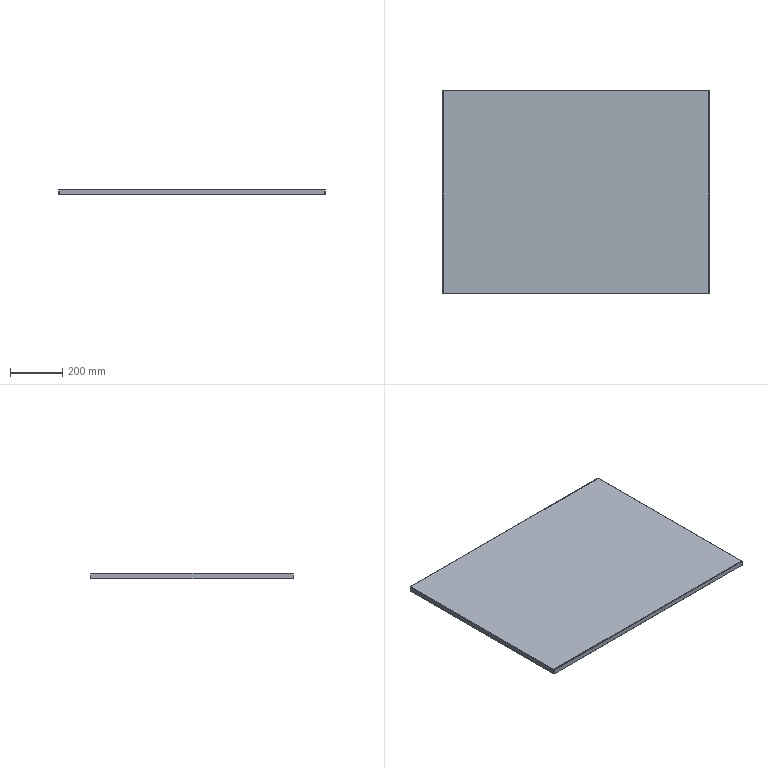Part | STEP file | X77-03016 | 1 solid | 38 faces | box 1018 x 778 x 20 mm | volume 1283744 mm3 | plane 22 | spline 8 | cylinder 8 | commonest cylinder face diameters 1.473 x4 4.473 x4
STEP:
#1=CARTESIAN_POINT('',(23.994,-5274.803,-1.5));
#2=VERTEX_POINT('',#1);
#3=CARTESIAN_POINT('',(1037.521,-5274.803,-1.5));
#4=VERTEX_POINT('',#3);
#5=CARTESIAN_POINT('',(23.964,-5274.803,-1.5));
#6=DIRECTION('',(1.,0.,0.));
#7=VECTOR('',#6,1000.);
#8=LINE('',#5,#7);
#9=EDGE_CURVE('',#2,#4,#8,.T.);
#10=ORIENTED_EDGE('',*,*,#9,.F.);
#11=CARTESIAN_POINT('',(23.994,-4501.276,-1.5));
#12=VERTEX_POINT('',#11);
#13=CARTESIAN_POINT('',(23.994,-4501.247,-1.5));
#14=DIRECTION('',(0.,-1.,0.));
#15=VECTOR('',#14,1000.);
#16=LINE('',#13,#15);
#17=EDGE_CURVE('',#12,#2,#16,.T.);
#18=ORIENTED_EDGE('',*,*,#17,.F.);
#19=CARTESIAN_POINT('',(1037.521,-4501.276,-1.5));
#20=VERTEX_POINT('',#19);
#21=CARTESIAN_POINT('',(1037.55,-4501.276,-1.5));
#22=DIRECTION('',(-1.,0.,0.));
#23=VECTOR('',#22,1000.);
#24=LINE('',#21,#23);
#25=EDGE_CURVE('',#20,#12,#24,.T.);
#26=ORIENTED_EDGE('',*,*,#25,.F.);
#27=CARTESIAN_POINT('',(1037.521,-5274.833,-1.5));
#28=DIRECTION('',(0.,1.,0.));
#29=VECTOR('',#28,1000.);
#30=LINE('',#27,#29);
#31=EDGE_CURVE('',#4,#20,#30,.T.);
#32=ORIENTED_EDGE('',*,*,#31,.F.);
#33=EDGE_LOOP('',(#10,#18,#26,#32));
#34=FACE_OUTER_BOUND('',#33,.T.);
#35=CARTESIAN_POINT('',(23.257,-5275.54,-1.5));
#36=DIRECTION('',(0.,0.,1.));
#37=DIRECTION('',(1.,0.,0.));
#38=AXIS2_PLACEMENT_3D('',#35,#36,#37);
#39=PLANE('',#38);
#40=ADVANCED_FACE('',(#34),#39,.F.);
#41=CARTESIAN_POINT('',(23.994,-4501.276,0.));
#42=VERTEX_POINT('',#41);
#43=CARTESIAN_POINT('',(23.994,-5274.803,0.));
#44=VERTEX_POINT('',#43);
#45=CARTESIAN_POINT('',(23.994,-4501.247,0.));
#46=DIRECTION('',(0.,-1.,0.));
#47=VECTOR('',#46,1000.);
#48=LINE('',#45,#47);
#49=EDGE_CURVE('',#42,#44,#48,.T.);
#50=ORIENTED_EDGE('',*,*,#49,.T.);
#51=CARTESIAN_POINT('',(1037.521,-5274.803,0.));
#52=VERTEX_POINT('',#51);
#53=CARTESIAN_POINT('',(23.964,-5274.803,0.));
#54=DIRECTION('',(1.,0.,0.));
#55=VECTOR('',#54,1000.);
#56=LINE('',#53,#55);
#57=EDGE_CURVE('',#44,#52,#56,.T.);
#58=ORIENTED_EDGE('',*,*,#57,.T.);
#59=CARTESIAN_POINT('',(1037.521,-4501.276,0.));
#60=VERTEX_POINT('',#59);
#61=CARTESIAN_POINT('',(1037.521,-5274.833,0.));
#62=DIRECTION('',(0.,1.,0.));
#63=VECTOR('',#62,1000.);
#64=LINE('',#61,#63);
#65=EDGE_CURVE('',#52,#60,#64,.T.);
#66=ORIENTED_EDGE('',*,*,#65,.T.);
#67=CARTESIAN_POINT('',(1037.55,-4501.276,0.));
#68=DIRECTION('',(-1.,0.,0.));
#69=VECTOR('',#68,1000.);
#70=LINE('',#67,#69);
#71=EDGE_CURVE('',#60,#42,#70,.T.);
#72=ORIENTED_EDGE('',*,*,#71,.T.);
#73=EDGE_LOOP('',(#50,#58,#66,#72));
#74=FACE_OUTER_BOUND('',#73,.T.);
#75=CARTESIAN_POINT('',(23.257,-5275.54,0.));
#76=DIRECTION('',(0.,0.,1.));
#77=DIRECTION('',(1.,0.,0.));
#78=AXIS2_PLACEMENT_3D('',#75,#76,#77);
#79=PLANE('',#78);
#80=ADVANCED_FACE('',(#74),#79,.T.);
#81=CARTESIAN_POINT('',(21.757,-5274.833,-2.237));
#82=VERTEX_POINT('',#81);
#83=CARTESIAN_POINT('',(23.257,-5274.833,-2.237));
#84=VERTEX_POINT('',#83);
#85=CARTESIAN_POINT('',(23.257,-5274.833,-2.237));
#86=DIRECTION('',(1.,0.,0.));
#87=VECTOR('',#86,1000.);
#88=LINE('',#85,#87);
#89=EDGE_CURVE('',#82,#84,#88,.T.);
#90=ORIENTED_EDGE('',*,*,#89,.T.);
#91=CARTESIAN_POINT('',(23.994,-5274.803,-1.5));
#92=CARTESIAN_POINT('',(23.801,-5274.808,-1.5));
#93=CARTESIAN_POINT('',(23.609,-5274.813,-1.579));
#94=CARTESIAN_POINT('',(23.337,-5274.823,-1.852));
#95=CARTESIAN_POINT('',(23.257,-5274.828,-2.044));
#96=CARTESIAN_POINT('',(23.257,-5274.833,-2.237));
#97=B_SPLINE_CURVE_WITH_KNOTS('',3,(#91,#92,#93,#94,#95,#96),.UNSPECIFIED.,.F.,.F.,(4,2,4),(0.,0.5,1.),.UNSPECIFIED.);
#98=EDGE_CURVE('',#2,#84,#97,.T.);
#99=ORIENTED_EDGE('',*,*,#98,.F.);
#100=CARTESIAN_POINT('',(23.994,-5274.803,-1.5));
#101=DIRECTION('',(0.,0.,1.));
#102=VECTOR('',#101,1000.);
#103=LINE('',#100,#102);
#104=EDGE_CURVE('',#2,#44,#103,.T.);
#105=ORIENTED_EDGE('',*,*,#104,.T.);
#106=CARTESIAN_POINT('',(23.994,-5274.803,0.));
#107=CARTESIAN_POINT('',(23.701,-5274.806,0.));
#108=CARTESIAN_POINT('',(23.408,-5274.808,-0.05821));
#109=CARTESIAN_POINT('',(22.867,-5274.813,-0.2823));
#110=CARTESIAN_POINT('',(22.619,-5274.815,-0.4481));
#111=CARTESIAN_POINT('',(22.205,-5274.82,-0.8621));
#112=CARTESIAN_POINT('',(22.04,-5274.823,-1.11));
#113=CARTESIAN_POINT('',(21.815,-5274.828,-1.651));
#114=CARTESIAN_POINT('',(21.757,-5274.83,-1.944));
#115=CARTESIAN_POINT('',(21.757,-5274.833,-2.237));
#116=B_SPLINE_CURVE_WITH_KNOTS('',3,(#106,#107,#108,#109,#110,#111,#112,#113,#114,#115),.UNSPECIFIED.,.F.,.F.,(4,2,2,2,4),(0.,0.25,0.5,0.75,1.),.UNSPECIFIED.);
#117=EDGE_CURVE('',#44,#82,#116,.T.);
#118=ORIENTED_EDGE('',*,*,#117,.T.);
#119=EDGE_LOOP('',(#90,#99,#105,#118));
#120=FACE_OUTER_BOUND('',#119,.T.);
#121=CARTESIAN_POINT('',(23.994,-5274.803,0.015));
#122=CARTESIAN_POINT('',(23.699,-5274.806,0.015));
#123=CARTESIAN_POINT('',(23.405,-5274.808,-0.0436));
#124=CARTESIAN_POINT('',(22.86,-5274.813,-0.2692));
#125=CARTESIAN_POINT('',(22.61,-5274.815,-0.4361));
#126=CARTESIAN_POINT('',(22.193,-5274.82,-0.8529));
#127=CARTESIAN_POINT('',(22.026,-5274.823,-1.103));
#128=CARTESIAN_POINT('',(21.801,-5274.828,-1.647));
#129=CARTESIAN_POINT('',(21.742,-5274.83,-1.942));
#130=CARTESIAN_POINT('',(21.742,-5274.833,-2.237));
#131=CARTESIAN_POINT('',(23.994,-5274.803,0.));
#132=CARTESIAN_POINT('',(23.701,-5274.806,0.));
#133=CARTESIAN_POINT('',(23.408,-5274.808,-0.05821));
#134=CARTESIAN_POINT('',(22.867,-5274.813,-0.2823));
#135=CARTESIAN_POINT('',(22.619,-5274.815,-0.4481));
#136=CARTESIAN_POINT('',(22.205,-5274.82,-0.8621));
#137=CARTESIAN_POINT('',(22.04,-5274.823,-1.11));
#138=CARTESIAN_POINT('',(21.815,-5274.828,-1.651));
#139=CARTESIAN_POINT('',(21.757,-5274.83,-1.944));
#140=CARTESIAN_POINT('',(21.757,-5274.833,-2.237));
#141=CARTESIAN_POINT('',(23.994,-5274.803,-1.5));
#142=CARTESIAN_POINT('',(23.897,-5274.806,-1.5));
#143=CARTESIAN_POINT('',(23.801,-5274.808,-1.519));
#144=CARTESIAN_POINT('',(23.623,-5274.813,-1.593));
#145=CARTESIAN_POINT('',(23.541,-5274.815,-1.648));
#146=CARTESIAN_POINT('',(23.405,-5274.82,-1.784));
#147=CARTESIAN_POINT('',(23.35,-5274.823,-1.866));
#148=CARTESIAN_POINT('',(23.276,-5274.828,-2.044));
#149=CARTESIAN_POINT('',(23.257,-5274.83,-2.14));
#150=CARTESIAN_POINT('',(23.257,-5274.833,-2.237));
#151=CARTESIAN_POINT('',(23.994,-5274.803,-1.515));
#152=CARTESIAN_POINT('',(23.899,-5274.806,-1.515));
#153=CARTESIAN_POINT('',(23.805,-5274.808,-1.534));
#154=CARTESIAN_POINT('',(23.631,-5274.813,-1.606));
#155=CARTESIAN_POINT('',(23.551,-5274.815,-1.66));
#156=CARTESIAN_POINT('',(23.417,-5274.82,-1.793));
#157=CARTESIAN_POINT('',(23.363,-5274.823,-1.873));
#158=CARTESIAN_POINT('',(23.291,-5274.828,-2.048));
#159=CARTESIAN_POINT('',(23.272,-5274.83,-2.142));
#160=CARTESIAN_POINT('',(23.272,-5274.833,-2.237));
#161=B_SPLINE_SURFACE_WITH_KNOTS('',1,3,((#121,#122,#123,#124,#125,#126,#127,#128,#129,#130),(#131,#132,#133,#134,#135,#136,#137,#138,#139,#140),(#141,#142,#143,#144,#145,#146,#147,#148,#149,#150),(#151,#152,#153,#154,#155,#156,#157,#158,#159,#160)),.UNSPECIFIED.,.F.,.F.,.F.,(2,1,1,2),(4,2,2,2,4),(-0.01,0.,1.,1.01),(0.,0.25,0.5,0.75,1.),.UNSPECIFIED.);
#162=ADVANCED_FACE('',(#120),#161,.F.);
#163=ORIENTED_EDGE('',*,*,#49,.F.);
#164=CARTESIAN_POINT('',(21.757,-4501.247,-2.237));
#165=VERTEX_POINT('',#164);
#166=CARTESIAN_POINT('',(21.757,-4501.247,-2.237));
#167=CARTESIAN_POINT('',(21.757,-4501.249,-1.944));
#168=CARTESIAN_POINT('',(21.815,-4501.252,-1.651));
#169=CARTESIAN_POINT('',(22.04,-4501.257,-1.11));
#170=CARTESIAN_POINT('',(22.205,-4501.259,-0.8621));
#171=CARTESIAN_POINT('',(22.619,-4501.264,-0.4481));
#172=CARTESIAN_POINT('',(22.867,-4501.266,-0.2823));
#173=CARTESIAN_POINT('',(23.408,-4501.271,-0.05821));
#174=CARTESIAN_POINT('',(23.701,-4501.274,0.));
#175=CARTESIAN_POINT('',(23.994,-4501.276,0.));
#176=B_SPLINE_CURVE_WITH_KNOTS('',3,(#166,#167,#168,#169,#170,#171,#172,#173,#174,#175),.UNSPECIFIED.,.F.,.F.,(4,2,2,2,4),(0.,0.25,0.5,0.75,1.),.UNSPECIFIED.);
#177=EDGE_CURVE('',#165,#42,#176,.T.);
#178=ORIENTED_EDGE('',*,*,#177,.F.);
#179=CARTESIAN_POINT('',(21.757,-4500.54,-2.237));
#180=DIRECTION('',(0.,1.,0.));
#181=VECTOR('',#180,1000.);
#182=LINE('',#179,#181);
#183=EDGE_CURVE('',#82,#165,#182,.T.);
#184=ORIENTED_EDGE('',*,*,#183,.F.);
#185=ORIENTED_EDGE('',*,*,#117,.F.);
#186=EDGE_LOOP('',(#163,#178,#184,#185));
#187=FACE_OUTER_BOUND('',#186,.T.);
#188=CARTESIAN_POINT('',(23.994,-4501.247,-2.237));
#189=DIRECTION('',(0.,1.,0.));
#190=DIRECTION('',(-1.,0.,0.));
#191=AXIS2_PLACEMENT_3D('',#188,#189,#190);
#192=CYLINDRICAL_SURFACE('',#191,2.237);
#193=ADVANCED_FACE('',(#187),#192,.T.);
#194=CARTESIAN_POINT('',(23.257,-4501.247,-2.237));
#195=VERTEX_POINT('',#194);
#196=CARTESIAN_POINT('',(23.257,-4501.247,-2.237));
#197=CARTESIAN_POINT('',(23.257,-4501.252,-2.044));
#198=CARTESIAN_POINT('',(23.337,-4501.257,-1.852));
#199=CARTESIAN_POINT('',(23.609,-4501.266,-1.579));
#200=CARTESIAN_POINT('',(23.801,-4501.271,-1.5));
#201=CARTESIAN_POINT('',(23.994,-4501.276,-1.5));
#202=B_SPLINE_CURVE_WITH_KNOTS('',3,(#196,#197,#198,#199,#200,#201),.UNSPECIFIED.,.F.,.F.,(4,2,4),(0.,0.5,1.),.UNSPECIFIED.);
#203=EDGE_CURVE('',#195,#12,#202,.T.);
#204=ORIENTED_EDGE('',*,*,#203,.F.);
#205=CARTESIAN_POINT('',(23.257,-4501.247,-2.237));
#206=DIRECTION('',(1.,0.,0.));
#207=VECTOR('',#206,1000.);
#208=LINE('',#205,#207);
#209=EDGE_CURVE('',#165,#195,#208,.T.);
#210=ORIENTED_EDGE('',*,*,#209,.F.);
#211=ORIENTED_EDGE('',*,*,#177,.T.);
#212=CARTESIAN_POINT('',(23.994,-4501.276,-1.5));
#213=DIRECTION('',(0.,0.,1.));
#214=VECTOR('',#213,1000.);
#215=LINE('',#212,#214);
#216=EDGE_CURVE('',#12,#42,#215,.T.);
#217=ORIENTED_EDGE('',*,*,#216,.F.);
#218=EDGE_LOOP('',(#204,#210,#211,#217));
#219=FACE_OUTER_BOUND('',#218,.T.);
#220=CARTESIAN_POINT('',(21.742,-4501.247,-2.237));
#221=CARTESIAN_POINT('',(21.742,-4501.249,-1.942));
#222=CARTESIAN_POINT('',(21.801,-4501.252,-1.647));
#223=CARTESIAN_POINT('',(22.026,-4501.257,-1.103));
#224=CARTESIAN_POINT('',(22.193,-4501.259,-0.8529));
#225=CARTESIAN_POINT('',(22.61,-4501.264,-0.4361));
#226=CARTESIAN_POINT('',(22.86,-4501.266,-0.2692));
#227=CARTESIAN_POINT('',(23.405,-4501.271,-0.0436));
#228=CARTESIAN_POINT('',(23.699,-4501.274,0.015));
#229=CARTESIAN_POINT('',(23.994,-4501.276,0.015));
#230=CARTESIAN_POINT('',(21.757,-4501.247,-2.237));
#231=CARTESIAN_POINT('',(21.757,-4501.249,-1.944));
#232=CARTESIAN_POINT('',(21.815,-4501.252,-1.651));
#233=CARTESIAN_POINT('',(22.04,-4501.257,-1.11));
#234=CARTESIAN_POINT('',(22.205,-4501.259,-0.8621));
#235=CARTESIAN_POINT('',(22.619,-4501.264,-0.4481));
#236=CARTESIAN_POINT('',(22.867,-4501.266,-0.2823));
#237=CARTESIAN_POINT('',(23.408,-4501.271,-0.05821));
#238=CARTESIAN_POINT('',(23.701,-4501.274,0.));
#239=CARTESIAN_POINT('',(23.994,-4501.276,0.));
#240=CARTESIAN_POINT('',(23.257,-4501.247,-2.237));
#241=CARTESIAN_POINT('',(23.257,-4501.249,-2.14));
#242=CARTESIAN_POINT('',(23.276,-4501.252,-2.044));
#243=CARTESIAN_POINT('',(23.35,-4501.257,-1.866));
#244=CARTESIAN_POINT('',(23.405,-4501.259,-1.784));
#245=CARTESIAN_POINT('',(23.541,-4501.264,-1.648));
#246=CARTESIAN_POINT('',(23.623,-4501.266,-1.593));
#247=CARTESIAN_POINT('',(23.801,-4501.271,-1.519));
#248=CARTESIAN_POINT('',(23.897,-4501.274,-1.5));
#249=CARTESIAN_POINT('',(23.994,-4501.276,-1.5));
#250=CARTESIAN_POINT('',(23.272,-4501.247,-2.237));
#251=CARTESIAN_POINT('',(23.272,-4501.249,-2.142));
#252=CARTESIAN_POINT('',(23.291,-4501.252,-2.048));
#253=CARTESIAN_POINT('',(23.363,-4501.257,-1.873));
#254=CARTESIAN_POINT('',(23.417,-4501.259,-1.793));
#255=CARTESIAN_POINT('',(23.551,-4501.264,-1.66));
#256=CARTESIAN_POINT('',(23.631,-4501.266,-1.606));
#257=CARTESIAN_POINT('',(23.805,-4501.271,-1.534));
#258=CARTESIAN_POINT('',(23.899,-4501.274,-1.515));
#259=CARTESIAN_POINT('',(23.994,-4501.276,-1.515));
#260=B_SPLINE_SURFACE_WITH_KNOTS('',1,3,((#220,#221,#222,#223,#224,#225,#226,#227,#228,#229),(#230,#231,#232,#233,#234,#235,#236,#237,#238,#239),(#240,#241,#242,#243,#244,#245,#246,#247,#248,#249),(#250,#251,#252,#253,#254,#255,#256,#257,#258,#259)),.UNSPECIFIED.,.F.,.F.,.F.,(2,1,1,2),(4,2,2,2,4),(-0.01,0.,1.,1.01),(0.,0.25,0.5,0.75,1.),.UNSPECIFIED.);
#261=ADVANCED_FACE('',(#219),#260,.F.);
#262=ORIENTED_EDGE('',*,*,#17,.T.);
#263=ORIENTED_EDGE('',*,*,#98,.T.);
#264=CARTESIAN_POINT('',(23.257,-5275.54,-2.237));
#265=DIRECTION('',(0.,1.,0.));
#266=VECTOR('',#265,1000.);
#267=LINE('',#264,#266);
#268=EDGE_CURVE('',#84,#195,#267,.T.);
#269=ORIENTED_EDGE('',*,*,#268,.T.);
#270=ORIENTED_EDGE('',*,*,#203,.T.);
#271=EDGE_LOOP('',(#262,#263,#269,#270));
#272=FACE_OUTER_BOUND('',#271,.T.);
#273=CARTESIAN_POINT('',(23.994,-4501.247,-2.237));
#274=DIRECTION('',(0.,1.,0.));
#275=DIRECTION('',(-1.,0.,0.));
#276=AXIS2_PLACEMENT_3D('',#273,#274,#275);
#277=CYLINDRICAL_SURFACE('',#276,0.7366);
#278=ADVANCED_FACE('',(#272),#277,.F.);
#279=CARTESIAN_POINT('',(23.257,-5274.833,-20.));
#280=VERTEX_POINT('',#279);
#281=CARTESIAN_POINT('',(21.757,-5274.833,-20.));
#282=VERTEX_POINT('',#281);
#283=CARTESIAN_POINT('',(21.757,-5274.833,-20.));
#284=DIRECTION('',(-1.,0.,0.));
#285=VECTOR('',#284,1000.);
#286=LINE('',#283,#285);
#287=EDGE_CURVE('',#280,#282,#286,.T.);
#288=ORIENTED_EDGE('',*,*,#287,.F.);
#289=CARTESIAN_POINT('',(23.257,-5274.833,-1.5));
#290=DIRECTION('',(0.,0.,-1.));
#291=VECTOR('',#290,1000.);
#292=LINE('',#289,#291);
#293=EDGE_CURVE('',#84,#280,#292,.T.);
#294=ORIENTED_EDGE('',*,*,#293,.F.);
#295=ORIENTED_EDGE('',*,*,#89,.F.);
#296=CARTESIAN_POINT('',(21.757,-5274.833,-1.5));
#297=DIRECTION('',(0.,0.,1.));
#298=VECTOR('',#297,1000.);
#299=LINE('',#296,#298);
#300=EDGE_CURVE('',#282,#82,#299,.T.);
#301=ORIENTED_EDGE('',*,*,#300,.F.);
#302=EDGE_LOOP('',(#288,#294,#295,#301));
#303=FACE_OUTER_BOUND('',#302,.T.);
#304=CARTESIAN_POINT('',(23.257,-5274.833,-1.5));
#305=DIRECTION('',(0.,-1.,0.));
#306=DIRECTION('',(0.,0.,-1.));
#307=AXIS2_PLACEMENT_3D('',#304,#305,#306);
#308=PLANE('',#307);
#309=ADVANCED_FACE('',(#303),#308,.T.);
#310=CARTESIAN_POINT('',(21.757,-4501.247,-20.));
#311=VERTEX_POINT('',#310);
#312=CARTESIAN_POINT('',(21.757,-4501.247,-1.5));
#313=DIRECTION('',(0.,0.,1.));
#314=VECTOR('',#313,1000.);
#315=LINE('',#312,#314);
#316=EDGE_CURVE('',#311,#165,#315,.T.);
#317=ORIENTED_EDGE('',*,*,#316,.F.);
#318=CARTESIAN_POINT('',(21.757,-4500.54,-20.));
#319=DIRECTION('',(0.,1.,0.));
#320=VECTOR('',#319,1000.);
#321=LINE('',#318,#320);
#322=EDGE_CURVE('',#282,#311,#321,.T.);
#323=ORIENTED_EDGE('',*,*,#322,.F.);
#324=ORIENTED_EDGE('',*,*,#300,.T.);
#325=ORIENTED_EDGE('',*,*,#183,.T.);
#326=EDGE_LOOP('',(#317,#323,#324,#325));
#327=FACE_OUTER_BOUND('',#326,.T.);
#328=CARTESIAN_POINT('',(21.757,-4500.54,-1.5));
#329=DIRECTION('',(-1.,0.,0.));
#330=DIRECTION('',(0.,0.,1.));
#331=AXIS2_PLACEMENT_3D('',#328,#329,#330);
#332=PLANE('',#331);
#333=ADVANCED_FACE('',(#327),#332,.T.);
#334=CARTESIAN_POINT('',(23.257,-4501.247,-20.));
#335=VERTEX_POINT('',#334);
#336=CARTESIAN_POINT('',(23.257,-4500.54,-20.));
#337=DIRECTION('',(0.,1.,0.));
#338=VECTOR('',#337,1000.);
#339=LINE('',#336,#338);
#340=EDGE_CURVE('',#280,#335,#339,.T.);
#341=ORIENTED_EDGE('',*,*,#340,.T.);
#342=CARTESIAN_POINT('',(23.257,-4501.247,-1.5));
#343=DIRECTION('',(0.,0.,-1.));
#344=VECTOR('',#343,1000.);
#345=LINE('',#342,#344);
#346=EDGE_CURVE('',#195,#335,#345,.T.);
#347=ORIENTED_EDGE('',*,*,#346,.F.);
#348=ORIENTED_EDGE('',*,*,#268,.F.);
#349=ORIENTED_EDGE('',*,*,#293,.T.);
#350=EDGE_LOOP('',(#341,#347,#348,#349));
#351=FACE_OUTER_BOUND('',#350,.T.);
#352=CARTESIAN_POINT('',(23.257,-4500.54,-1.5));
#353=DIRECTION('',(-1.,0.,0.));
#354=DIRECTION('',(0.,0.,1.));
#355=AXIS2_PLACEMENT_3D('',#352,#353,#354);
#356=PLANE('',#355);
#357=ADVANCED_FACE('',(#351),#356,.F.);
#358=CARTESIAN_POINT('',(21.757,-4501.247,-20.));
#359=DIRECTION('',(-1.,0.,0.));
#360=VECTOR('',#359,1000.);
#361=LINE('',#358,#360);
#362=EDGE_CURVE('',#335,#311,#361,.T.);
#363=ORIENTED_EDGE('',*,*,#362,.F.);
#364=ORIENTED_EDGE('',*,*,#340,.F.);
#365=ORIENTED_EDGE('',*,*,#287,.T.);
#366=ORIENTED_EDGE('',*,*,#322,.T.);
#367=EDGE_LOOP('',(#363,#364,#365,#366));
#368=FACE_OUTER_BOUND('',#367,.T.);
#369=CARTESIAN_POINT('',(21.757,-4500.54,-20.));
#370=DIRECTION('',(0.,0.,-1.));
#371=DIRECTION('',(-1.,0.,0.));
#372=AXIS2_PLACEMENT_3D('',#369,#370,#371);
#373=PLANE('',#372);
#374=ADVANCED_FACE('',(#368),#373,.T.);
#375=ORIENTED_EDGE('',*,*,#346,.T.);
#376=ORIENTED_EDGE('',*,*,#362,.T.);
#377=ORIENTED_EDGE('',*,*,#316,.T.);
#378=ORIENTED_EDGE('',*,*,#209,.T.);
#379=EDGE_LOOP('',(#375,#376,#377,#378));
#380=FACE_OUTER_BOUND('',#379,.T.);
#381=CARTESIAN_POINT('',(23.257,-4501.247,-1.5));
#382=DIRECTION('',(0.,-1.,0.));
#383=DIRECTION('',(0.,0.,-1.));
#384=AXIS2_PLACEMENT_3D('',#381,#382,#383);
#385=PLANE('',#384);
#386=ADVANCED_FACE('',(#380),#385,.F.);
#387=CARTESIAN_POINT('',(23.964,-4499.04,-2.237));
#388=VERTEX_POINT('',#387);
#389=CARTESIAN_POINT('',(23.964,-4500.54,-2.237));
#390=VERTEX_POINT('',#389);
#391=CARTESIAN_POINT('',(23.964,-4500.54,-2.237));
#392=DIRECTION('',(0.,-1.,0.));
#393=VECTOR('',#392,1000.);
#394=LINE('',#391,#393);
#395=EDGE_CURVE('',#388,#390,#394,.T.);
#396=ORIENTED_EDGE('',*,*,#395,.T.);
#397=CARTESIAN_POINT('',(23.994,-4501.276,-1.5));
#398=CARTESIAN_POINT('',(23.989,-4501.083,-1.5));
#399=CARTESIAN_POINT('',(23.984,-4500.892,-1.579));
#400=CARTESIAN_POINT('',(23.974,-4500.619,-1.852));
#401=CARTESIAN_POINT('',(23.969,-4500.54,-2.044));
#402=CARTESIAN_POINT('',(23.964,-4500.54,-2.237));
#403=B_SPLINE_CURVE_WITH_KNOTS('',3,(#397,#398,#399,#400,#401,#402),.UNSPECIFIED.,.F.,.F.,(4,2,4),(0.,0.5,1.),.UNSPECIFIED.);
#404=EDGE_CURVE('',#12,#390,#403,.T.);
#405=ORIENTED_EDGE('',*,*,#404,.F.);
#406=ORIENTED_EDGE('',*,*,#216,.T.);
#407=CARTESIAN_POINT('',(23.994,-4501.276,0.));
#408=CARTESIAN_POINT('',(23.991,-4500.983,0.));
#409=CARTESIAN_POINT('',(23.989,-4500.691,-0.05821));
#410=CARTESIAN_POINT('',(23.984,-4500.15,-0.2823));
#411=CARTESIAN_POINT('',(23.982,-4499.902,-0.4481));
#412=CARTESIAN_POINT('',(23.977,-4499.488,-0.8621));
#413=CARTESIAN_POINT('',(23.974,-4499.322,-1.11));
#414=CARTESIAN_POINT('',(23.969,-4499.098,-1.651));
#415=CARTESIAN_POINT('',(23.967,-4499.04,-1.944));
#416=CARTESIAN_POINT('',(23.964,-4499.04,-2.237));
#417=B_SPLINE_CURVE_WITH_KNOTS('',3,(#407,#408,#409,#410,#411,#412,#413,#414,#415,#416),.UNSPECIFIED.,.F.,.F.,(4,2,2,2,4),(0.,0.25,0.5,0.75,1.),.UNSPECIFIED.);
#418=EDGE_CURVE('',#42,#388,#417,.T.);
#419=ORIENTED_EDGE('',*,*,#418,.T.);
#420=EDGE_LOOP('',(#396,#405,#406,#419));
#421=FACE_OUTER_BOUND('',#420,.T.);
#422=CARTESIAN_POINT('',(23.994,-4501.276,0.015));
#423=CARTESIAN_POINT('',(23.991,-4500.981,0.015));
#424=CARTESIAN_POINT('',(23.989,-4500.687,-0.0436));
#425=CARTESIAN_POINT('',(23.984,-4500.142,-0.2692));
#426=CARTESIAN_POINT('',(23.982,-4499.893,-0.4361));
#427=CARTESIAN_POINT('',(23.977,-4499.476,-0.8529));
#428=CARTESIAN_POINT('',(23.974,-4499.309,-1.103));
#429=CARTESIAN_POINT('',(23.969,-4499.083,-1.647));
#430=CARTESIAN_POINT('',(23.967,-4499.025,-1.942));
#431=CARTESIAN_POINT('',(23.964,-4499.025,-2.237));
#432=CARTESIAN_POINT('',(23.994,-4501.276,0.));
#433=CARTESIAN_POINT('',(23.991,-4500.983,0.));
#434=CARTESIAN_POINT('',(23.989,-4500.691,-0.05821));
#435=CARTESIAN_POINT('',(23.984,-4500.15,-0.2823));
#436=CARTESIAN_POINT('',(23.982,-4499.902,-0.4481));
#437=CARTESIAN_POINT('',(23.977,-4499.488,-0.8621));
#438=CARTESIAN_POINT('',(23.974,-4499.322,-1.11));
#439=CARTESIAN_POINT('',(23.969,-4499.098,-1.651));
#440=CARTESIAN_POINT('',(23.967,-4499.04,-1.944));
#441=CARTESIAN_POINT('',(23.964,-4499.04,-2.237));
#442=CARTESIAN_POINT('',(23.994,-4501.276,-1.5));
#443=CARTESIAN_POINT('',(23.991,-4501.18,-1.5));
#444=CARTESIAN_POINT('',(23.989,-4501.083,-1.519));
#445=CARTESIAN_POINT('',(23.984,-4500.905,-1.593));
#446=CARTESIAN_POINT('',(23.982,-4500.824,-1.648));
#447=CARTESIAN_POINT('',(23.977,-4500.687,-1.784));
#448=CARTESIAN_POINT('',(23.974,-4500.633,-1.866));
#449=CARTESIAN_POINT('',(23.969,-4500.559,-2.044));
#450=CARTESIAN_POINT('',(23.967,-4500.54,-2.14));
#451=CARTESIAN_POINT('',(23.964,-4500.54,-2.237));
#452=CARTESIAN_POINT('',(23.994,-4501.276,-1.515));
#453=CARTESIAN_POINT('',(23.991,-4501.182,-1.515));
#454=CARTESIAN_POINT('',(23.989,-4501.087,-1.534));
#455=CARTESIAN_POINT('',(23.984,-4500.913,-1.606));
#456=CARTESIAN_POINT('',(23.982,-4500.833,-1.66));
#457=CARTESIAN_POINT('',(23.977,-4500.699,-1.793));
#458=CARTESIAN_POINT('',(23.974,-4500.646,-1.873));
#459=CARTESIAN_POINT('',(23.969,-4500.574,-2.048));
#460=CARTESIAN_POINT('',(23.967,-4500.555,-2.142));
#461=CARTESIAN_POINT('',(23.964,-4500.555,-2.237));
#462=B_SPLINE_SURFACE_WITH_KNOTS('',1,3,((#422,#423,#424,#425,#426,#427,#428,#429,#430,#431),(#432,#433,#434,#435,#436,#437,#438,#439,#440,#441),(#442,#443,#444,#445,#446,#447,#448,#449,#450,#451),(#452,#453,#454,#455,#456,#457,#458,#459,#460,#461)),.UNSPECIFIED.,.F.,.F.,.F.,(2,1,1,2),(4,2,2,2,4),(-0.01,0.,1.,1.01),(0.,0.25,0.5,0.75,1.),.UNSPECIFIED.);
#463=ADVANCED_FACE('',(#421),#462,.F.);
#464=ORIENTED_EDGE('',*,*,#71,.F.);
#465=CARTESIAN_POINT('',(1037.55,-4499.04,-2.237));
#466=VERTEX_POINT('',#465);
#467=CARTESIAN_POINT('',(1037.55,-4499.04,-2.237));
#468=CARTESIAN_POINT('',(1037.548,-4499.04,-1.944));
#469=CARTESIAN_POINT('',(1037.545,-4499.098,-1.651));
#470=CARTESIAN_POINT('',(1037.54,-4499.322,-1.11));
#471=CARTESIAN_POINT('',(1037.538,-4499.488,-0.8621));
#472=CARTESIAN_POINT('',(1037.533,-4499.902,-0.4481));
#473=CARTESIAN_POINT('',(1037.531,-4500.15,-0.2823));
#474=CARTESIAN_POINT('',(1037.526,-4500.691,-0.05821));
#475=CARTESIAN_POINT('',(1037.523,-4500.983,0.));
#476=CARTESIAN_POINT('',(1037.521,-4501.276,0.));
#477=B_SPLINE_CURVE_WITH_KNOTS('',3,(#467,#468,#469,#470,#471,#472,#473,#474,#475,#476),.UNSPECIFIED.,.F.,.F.,(4,2,2,2,4),(0.,0.25,0.5,0.75,1.),.UNSPECIFIED.);
#478=EDGE_CURVE('',#466,#60,#477,.T.);
#479=ORIENTED_EDGE('',*,*,#478,.F.);
#480=CARTESIAN_POINT('',(1038.257,-4499.04,-2.237));
#481=DIRECTION('',(-1.,0.,0.));
#482=VECTOR('',#481,1000.);
#483=LINE('',#480,#482);
#484=EDGE_CURVE('',#466,#388,#483,.T.);
#485=ORIENTED_EDGE('',*,*,#484,.T.);
#486=ORIENTED_EDGE('',*,*,#418,.F.);
#487=EDGE_LOOP('',(#464,#479,#485,#486));
#488=FACE_OUTER_BOUND('',#487,.T.);
#489=CARTESIAN_POINT('',(1037.55,-4501.276,-2.237));
#490=DIRECTION('',(1.,0.,0.));
#491=DIRECTION('',(0.,1.,0.));
#492=AXIS2_PLACEMENT_3D('',#489,#490,#491);
#493=CYLINDRICAL_SURFACE('',#492,2.237);
#494=ADVANCED_FACE('',(#488),#493,.T.);
#495=CARTESIAN_POINT('',(1037.55,-4500.54,-2.237));
#496=VERTEX_POINT('',#495);
#497=CARTESIAN_POINT('',(1037.55,-4500.54,-2.237));
#498=CARTESIAN_POINT('',(1037.545,-4500.54,-2.044));
#499=CARTESIAN_POINT('',(1037.54,-4500.619,-1.852));
#500=CARTESIAN_POINT('',(1037.531,-4500.892,-1.579));
#501=CARTESIAN_POINT('',(1037.526,-4501.083,-1.5));
#502=CARTESIAN_POINT('',(1037.521,-4501.276,-1.5));
#503=B_SPLINE_CURVE_WITH_KNOTS('',3,(#497,#498,#499,#500,#501,#502),.UNSPECIFIED.,.F.,.F.,(4,2,4),(0.,0.5,1.),.UNSPECIFIED.);
#504=EDGE_CURVE('',#496,#20,#503,.T.);
#505=ORIENTED_EDGE('',*,*,#504,.F.);
#506=CARTESIAN_POINT('',(1037.55,-4500.54,-2.237));
#507=DIRECTION('',(0.,-1.,0.));
#508=VECTOR('',#507,1000.);
#509=LINE('',#506,#508);
#510=EDGE_CURVE('',#466,#496,#509,.T.);
#511=ORIENTED_EDGE('',*,*,#510,.F.);
#512=ORIENTED_EDGE('',*,*,#478,.T.);
#513=CARTESIAN_POINT('',(1037.521,-4501.276,-1.5));
#514=DIRECTION('',(0.,0.,1.));
#515=VECTOR('',#514,1000.);
#516=LINE('',#513,#515);
#517=EDGE_CURVE('',#20,#60,#516,.T.);
#518=ORIENTED_EDGE('',*,*,#517,.F.);
#519=EDGE_LOOP('',(#505,#511,#512,#518));
#520=FACE_OUTER_BOUND('',#519,.T.);
#521=CARTESIAN_POINT('',(1037.55,-4499.025,-2.237));
#522=CARTESIAN_POINT('',(1037.548,-4499.025,-1.942));
#523=CARTESIAN_POINT('',(1037.545,-4499.083,-1.647));
#524=CARTESIAN_POINT('',(1037.54,-4499.309,-1.103));
#525=CARTESIAN_POINT('',(1037.538,-4499.476,-0.8529));
#526=CARTESIAN_POINT('',(1037.533,-4499.893,-0.4361));
#527=CARTESIAN_POINT('',(1037.531,-4500.142,-0.2692));
#528=CARTESIAN_POINT('',(1037.526,-4500.687,-0.0436));
#529=CARTESIAN_POINT('',(1037.523,-4500.981,0.015));
#530=CARTESIAN_POINT('',(1037.521,-4501.276,0.015));
#531=CARTESIAN_POINT('',(1037.55,-4499.04,-2.237));
#532=CARTESIAN_POINT('',(1037.548,-4499.04,-1.944));
#533=CARTESIAN_POINT('',(1037.545,-4499.098,-1.651));
#534=CARTESIAN_POINT('',(1037.54,-4499.322,-1.11));
#535=CARTESIAN_POINT('',(1037.538,-4499.488,-0.8621));
#536=CARTESIAN_POINT('',(1037.533,-4499.902,-0.4481));
#537=CARTESIAN_POINT('',(1037.531,-4500.15,-0.2823));
#538=CARTESIAN_POINT('',(1037.526,-4500.691,-0.05821));
#539=CARTESIAN_POINT('',(1037.523,-4500.983,0.));
#540=CARTESIAN_POINT('',(1037.521,-4501.276,0.));
#541=CARTESIAN_POINT('',(1037.55,-4500.54,-2.237));
#542=CARTESIAN_POINT('',(1037.548,-4500.54,-2.14));
#543=CARTESIAN_POINT('',(1037.545,-4500.559,-2.044));
#544=CARTESIAN_POINT('',(1037.54,-4500.633,-1.866));
#545=CARTESIAN_POINT('',(1037.538,-4500.687,-1.784));
#546=CARTESIAN_POINT('',(1037.533,-4500.824,-1.648));
#547=CARTESIAN_POINT('',(1037.531,-4500.905,-1.593));
#548=CARTESIAN_POINT('',(1037.526,-4501.083,-1.519));
#549=CARTESIAN_POINT('',(1037.523,-4501.18,-1.5));
#550=CARTESIAN_POINT('',(1037.521,-4501.276,-1.5));
#551=CARTESIAN_POINT('',(1037.55,-4500.555,-2.237));
#552=CARTESIAN_POINT('',(1037.548,-4500.555,-2.142));
#553=CARTESIAN_POINT('',(1037.545,-4500.574,-2.048));
#554=CARTESIAN_POINT('',(1037.54,-4500.646,-1.873));
#555=CARTESIAN_POINT('',(1037.538,-4500.699,-1.793));
#556=CARTESIAN_POINT('',(1037.533,-4500.833,-1.66));
#557=CARTESIAN_POINT('',(1037.531,-4500.913,-1.606));
#558=CARTESIAN_POINT('',(1037.526,-4501.087,-1.534));
#559=CARTESIAN_POINT('',(1037.523,-4501.182,-1.515));
#560=CARTESIAN_POINT('',(1037.521,-4501.276,-1.515));
#561=B_SPLINE_SURFACE_WITH_KNOTS('',1,3,((#521,#522,#523,#524,#525,#526,#527,#528,#529,#530),(#531,#532,#533,#534,#535,#536,#537,#538,#539,#540),(#541,#542,#543,#544,#545,#546,#547,#548,#549,#550),(#551,#552,#553,#554,#555,#556,#557,#558,#559,#560)),.UNSPECIFIED.,.F.,.F.,.F.,(2,1,1,2),(4,2,2,2,4),(-0.01,0.,1.,1.01),(0.,0.25,0.5,0.75,1.),.UNSPECIFIED.);
#562=ADVANCED_FACE('',(#520),#561,.F.);
#563=ORIENTED_EDGE('',*,*,#25,.T.);
#564=ORIENTED_EDGE('',*,*,#404,.T.);
#565=CARTESIAN_POINT('',(23.257,-4500.54,-2.237));
#566=DIRECTION('',(1.,0.,0.));
#567=VECTOR('',#566,1000.);
#568=LINE('',#565,#567);
#569=EDGE_CURVE('',#390,#496,#568,.T.);
#570=ORIENTED_EDGE('',*,*,#569,.T.);
#571=ORIENTED_EDGE('',*,*,#504,.T.);
#572=EDGE_LOOP('',(#563,#564,#570,#571));
#573=FACE_OUTER_BOUND('',#572,.T.);
#574=CARTESIAN_POINT('',(1037.55,-4501.276,-2.237));
#575=DIRECTION('',(1.,0.,0.));
#576=DIRECTION('',(0.,1.,0.));
#577=AXIS2_PLACEMENT_3D('',#574,#575,#576);
#578=CYLINDRICAL_SURFACE('',#577,0.7366);
#579=ADVANCED_FACE('',(#573),#578,.F.);
#580=CARTESIAN_POINT('',(23.964,-4500.54,-20.));
#581=VERTEX_POINT('',#580);
#582=CARTESIAN_POINT('',(23.964,-4499.04,-20.));
#583=VERTEX_POINT('',#582);
#584=CARTESIAN_POINT('',(23.964,-4499.04,-20.));
#585=DIRECTION('',(0.,1.,0.));
#586=VECTOR('',#585,1000.);
#587=LINE('',#584,#586);
#588=EDGE_CURVE('',#581,#583,#587,.T.);
#589=ORIENTED_EDGE('',*,*,#588,.F.);
#590=CARTESIAN_POINT('',(23.964,-4500.54,-1.5));
#591=DIRECTION('',(0.,0.,-1.));
#592=VECTOR('',#591,1000.);
#593=LINE('',#590,#592);
#594=EDGE_CURVE('',#390,#581,#593,.T.);
#595=ORIENTED_EDGE('',*,*,#594,.F.);
#596=ORIENTED_EDGE('',*,*,#395,.F.);
#597=CARTESIAN_POINT('',(23.964,-4499.04,-1.5));
#598=DIRECTION('',(0.,0.,-1.));
#599=VECTOR('',#598,1000.);
#600=LINE('',#597,#599);
#601=EDGE_CURVE('',#388,#583,#600,.T.);
#602=ORIENTED_EDGE('',*,*,#601,.T.);
#603=EDGE_LOOP('',(#589,#595,#596,#602));
#604=FACE_OUTER_BOUND('',#603,.T.);
#605=CARTESIAN_POINT('',(23.964,-4500.54,-1.5));
#606=DIRECTION('',(-1.,0.,0.));
#607=DIRECTION('',(0.,0.,1.));
#608=AXIS2_PLACEMENT_3D('',#605,#606,#607);
#609=PLANE('',#608);
#610=ADVANCED_FACE('',(#604),#609,.T.);
#611=ORIENTED_EDGE('',*,*,#484,.F.);
#612=CARTESIAN_POINT('',(1037.55,-4499.04,-20.));
#613=VERTEX_POINT('',#612);
#614=CARTESIAN_POINT('',(1037.55,-4499.04,-1.5));
#615=DIRECTION('',(0.,0.,-1.));
#616=VECTOR('',#615,1000.);
#617=LINE('',#614,#616);
#618=EDGE_CURVE('',#466,#613,#617,.T.);
#619=ORIENTED_EDGE('',*,*,#618,.T.);
#620=CARTESIAN_POINT('',(23.257,-4499.04,-20.));
#621=DIRECTION('',(1.,0.,0.));
#622=VECTOR('',#621,1000.);
#623=LINE('',#620,#622);
#624=EDGE_CURVE('',#583,#613,#623,.T.);
#625=ORIENTED_EDGE('',*,*,#624,.F.);
#626=ORIENTED_EDGE('',*,*,#601,.F.);
#627=EDGE_LOOP('',(#611,#619,#625,#626));
#628=FACE_OUTER_BOUND('',#627,.T.);
#629=CARTESIAN_POINT('',(1038.257,-4499.04,-1.5));
#630=DIRECTION('',(0.,-1.,0.));
#631=DIRECTION('',(0.,0.,-1.));
#632=AXIS2_PLACEMENT_3D('',#629,#630,#631);
#633=PLANE('',#632);
#634=ADVANCED_FACE('',(#628),#633,.F.);
#635=CARTESIAN_POINT('',(1037.55,-4500.54,-20.));
#636=VERTEX_POINT('',#635);
#637=CARTESIAN_POINT('',(1037.55,-4500.54,-1.5));
#638=DIRECTION('',(0.,0.,-1.));
#639=VECTOR('',#638,1000.);
#640=LINE('',#637,#639);
#641=EDGE_CURVE('',#496,#636,#640,.T.);
#642=ORIENTED_EDGE('',*,*,#641,.F.);
#643=ORIENTED_EDGE('',*,*,#569,.F.);
#644=ORIENTED_EDGE('',*,*,#594,.T.);
#645=CARTESIAN_POINT('',(23.257,-4500.54,-20.));
#646=DIRECTION('',(1.,0.,0.));
#647=VECTOR('',#646,1000.);
#648=LINE('',#645,#647);
#649=EDGE_CURVE('',#581,#636,#648,.T.);
#650=ORIENTED_EDGE('',*,*,#649,.T.);
#651=EDGE_LOOP('',(#642,#643,#644,#650));
#652=FACE_OUTER_BOUND('',#651,.T.);
#653=CARTESIAN_POINT('',(1038.257,-4500.54,-1.5));
#654=DIRECTION('',(0.,-1.,0.));
#655=DIRECTION('',(0.,0.,-1.));
#656=AXIS2_PLACEMENT_3D('',#653,#654,#655);
#657=PLANE('',#656);
#658=ADVANCED_FACE('',(#652),#657,.T.);
#659=CARTESIAN_POINT('',(1037.55,-4499.04,-20.));
#660=DIRECTION('',(0.,1.,0.));
#661=VECTOR('',#660,1000.);
#662=LINE('',#659,#661);
#663=EDGE_CURVE('',#636,#613,#662,.T.);
#664=ORIENTED_EDGE('',*,*,#663,.F.);
#665=ORIENTED_EDGE('',*,*,#649,.F.);
#666=ORIENTED_EDGE('',*,*,#588,.T.);
#667=ORIENTED_EDGE('',*,*,#624,.T.);
#668=EDGE_LOOP('',(#664,#665,#666,#667));
#669=FACE_OUTER_BOUND('',#668,.T.);
#670=CARTESIAN_POINT('',(23.257,-4499.04,-20.));
#671=DIRECTION('',(0.,0.,-1.));
#672=DIRECTION('',(0.,1.,0.));
#673=AXIS2_PLACEMENT_3D('',#670,#671,#672);
#674=PLANE('',#673);
#675=ADVANCED_FACE('',(#669),#674,.T.);
#676=ORIENTED_EDGE('',*,*,#641,.T.);
#677=ORIENTED_EDGE('',*,*,#663,.T.);
#678=ORIENTED_EDGE('',*,*,#618,.F.);
#679=ORIENTED_EDGE('',*,*,#510,.T.);
#680=EDGE_LOOP('',(#676,#677,#678,#679));
#681=FACE_OUTER_BOUND('',#680,.T.);
#682=CARTESIAN_POINT('',(1037.55,-4500.54,-1.5));
#683=DIRECTION('',(-1.,0.,0.));
#684=DIRECTION('',(0.,0.,1.));
#685=AXIS2_PLACEMENT_3D('',#682,#683,#684);
#686=PLANE('',#685);
#687=ADVANCED_FACE('',(#681),#686,.F.);
#688=CARTESIAN_POINT('',(1039.757,-4501.247,-2.237));
#689=VERTEX_POINT('',#688);
#690=CARTESIAN_POINT('',(1038.257,-4501.247,-2.237));
#691=VERTEX_POINT('',#690);
#692=CARTESIAN_POINT('',(1038.257,-4501.247,-2.237));
#693=DIRECTION('',(-1.,0.,0.));
#694=VECTOR('',#693,1000.);
#695=LINE('',#692,#694);
#696=EDGE_CURVE('',#689,#691,#695,.T.);
#697=ORIENTED_EDGE('',*,*,#696,.T.);
#698=CARTESIAN_POINT('',(1037.521,-4501.276,-1.5));
#699=CARTESIAN_POINT('',(1037.714,-4501.271,-1.5));
#700=CARTESIAN_POINT('',(1037.905,-4501.266,-1.579));
#701=CARTESIAN_POINT('',(1038.178,-4501.257,-1.852));
#702=CARTESIAN_POINT('',(1038.257,-4501.252,-2.044));
#703=CARTESIAN_POINT('',(1038.257,-4501.247,-2.237));
#704=B_SPLINE_CURVE_WITH_KNOTS('',3,(#698,#699,#700,#701,#702,#703),.UNSPECIFIED.,.F.,.F.,(4,2,4),(0.,0.5,1.),.UNSPECIFIED.);
#705=EDGE_CURVE('',#20,#691,#704,.T.);
#706=ORIENTED_EDGE('',*,*,#705,.F.);
#707=ORIENTED_EDGE('',*,*,#517,.T.);
#708=CARTESIAN_POINT('',(1037.521,-4501.276,0.));
#709=CARTESIAN_POINT('',(1037.813,-4501.274,0.));
#710=CARTESIAN_POINT('',(1038.106,-4501.271,-0.05821));
#711=CARTESIAN_POINT('',(1038.647,-4501.266,-0.2823));
#712=CARTESIAN_POINT('',(1038.895,-4501.264,-0.4481));
#713=CARTESIAN_POINT('',(1039.309,-4501.259,-0.8621));
#714=CARTESIAN_POINT('',(1039.475,-4501.257,-1.11));
#715=CARTESIAN_POINT('',(1039.699,-4501.252,-1.651));
#716=CARTESIAN_POINT('',(1039.757,-4501.249,-1.944));
#717=CARTESIAN_POINT('',(1039.757,-4501.247,-2.237));
#718=B_SPLINE_CURVE_WITH_KNOTS('',3,(#708,#709,#710,#711,#712,#713,#714,#715,#716,#717),.UNSPECIFIED.,.F.,.F.,(4,2,2,2,4),(0.,0.25,0.5,0.75,1.),.UNSPECIFIED.);
#719=EDGE_CURVE('',#60,#689,#718,.T.);
#720=ORIENTED_EDGE('',*,*,#719,.T.);
#721=EDGE_LOOP('',(#697,#706,#707,#720));
#722=FACE_OUTER_BOUND('',#721,.T.);
#723=CARTESIAN_POINT('',(1037.521,-4501.276,0.015));
#724=CARTESIAN_POINT('',(1037.815,-4501.274,0.015));
#725=CARTESIAN_POINT('',(1038.11,-4501.271,-0.0436));
#726=CARTESIAN_POINT('',(1038.655,-4501.266,-0.2692));
#727=CARTESIAN_POINT('',(1038.904,-4501.264,-0.4361));
#728=CARTESIAN_POINT('',(1039.321,-4501.259,-0.8529));
#729=CARTESIAN_POINT('',(1039.488,-4501.257,-1.103));
#730=CARTESIAN_POINT('',(1039.714,-4501.252,-1.647));
#731=CARTESIAN_POINT('',(1039.772,-4501.249,-1.942));
#732=CARTESIAN_POINT('',(1039.772,-4501.247,-2.237));
#733=CARTESIAN_POINT('',(1037.521,-4501.276,0.));
#734=CARTESIAN_POINT('',(1037.814,-4501.274,0.));
#735=CARTESIAN_POINT('',(1038.106,-4501.271,-0.05821));
#736=CARTESIAN_POINT('',(1038.647,-4501.266,-0.2823));
#737=CARTESIAN_POINT('',(1038.895,-4501.264,-0.4481));
#738=CARTESIAN_POINT('',(1039.309,-4501.259,-0.8621));
#739=CARTESIAN_POINT('',(1039.475,-4501.257,-1.11));
#740=CARTESIAN_POINT('',(1039.699,-4501.252,-1.651));
#741=CARTESIAN_POINT('',(1039.757,-4501.249,-1.944));
#742=CARTESIAN_POINT('',(1039.757,-4501.247,-2.237));
#743=CARTESIAN_POINT('',(1037.521,-4501.276,-1.5));
#744=CARTESIAN_POINT('',(1037.617,-4501.274,-1.5));
#745=CARTESIAN_POINT('',(1037.713,-4501.271,-1.519));
#746=CARTESIAN_POINT('',(1037.892,-4501.266,-1.593));
#747=CARTESIAN_POINT('',(1037.973,-4501.264,-1.648));
#748=CARTESIAN_POINT('',(1038.11,-4501.259,-1.784));
#749=CARTESIAN_POINT('',(1038.164,-4501.257,-1.866));
#750=CARTESIAN_POINT('',(1038.238,-4501.252,-2.044));
#751=CARTESIAN_POINT('',(1038.257,-4501.249,-2.14));
#752=CARTESIAN_POINT('',(1038.257,-4501.247,-2.237));
#753=CARTESIAN_POINT('',(1037.521,-4501.276,-1.515));
#754=CARTESIAN_POINT('',(1037.615,-4501.274,-1.515));
#755=CARTESIAN_POINT('',(1037.71,-4501.271,-1.534));
#756=CARTESIAN_POINT('',(1037.884,-4501.266,-1.606));
#757=CARTESIAN_POINT('',(1037.964,-4501.264,-1.66));
#758=CARTESIAN_POINT('',(1038.098,-4501.259,-1.793));
#759=CARTESIAN_POINT('',(1038.151,-4501.257,-1.873));
#760=CARTESIAN_POINT('',(1038.223,-4501.252,-2.048));
#761=CARTESIAN_POINT('',(1038.242,-4501.249,-2.142));
#762=CARTESIAN_POINT('',(1038.242,-4501.247,-2.237));
#763=B_SPLINE_SURFACE_WITH_KNOTS('',1,3,((#723,#724,#725,#726,#727,#728,#729,#730,#731,#732),(#733,#734,#735,#736,#737,#738,#739,#740,#741,#742),(#743,#744,#745,#746,#747,#748,#749,#750,#751,#752),(#753,#754,#755,#756,#757,#758,#759,#760,#761,#762)),.UNSPECIFIED.,.F.,.F.,.F.,(2,1,1,2),(4,2,2,2,4),(-0.01,0.,1.,1.01),(0.,0.25,0.5,0.75,1.),.UNSPECIFIED.);
#764=ADVANCED_FACE('',(#722),#763,.F.);
#765=ORIENTED_EDGE('',*,*,#65,.F.);
#766=CARTESIAN_POINT('',(1039.757,-5274.833,-2.237));
#767=VERTEX_POINT('',#766);
#768=CARTESIAN_POINT('',(1039.757,-5274.833,-2.237));
#769=CARTESIAN_POINT('',(1039.757,-5274.83,-1.944));
#770=CARTESIAN_POINT('',(1039.699,-5274.828,-1.651));
#771=CARTESIAN_POINT('',(1039.475,-5274.823,-1.11));
#772=CARTESIAN_POINT('',(1039.309,-5274.82,-0.8621));
#773=CARTESIAN_POINT('',(1038.895,-5274.815,-0.4481));
#774=CARTESIAN_POINT('',(1038.647,-5274.813,-0.2823));
#775=CARTESIAN_POINT('',(1038.106,-5274.808,-0.05821));
#776=CARTESIAN_POINT('',(1037.813,-5274.806,0.));
#777=CARTESIAN_POINT('',(1037.521,-5274.803,0.));
#778=B_SPLINE_CURVE_WITH_KNOTS('',3,(#768,#769,#770,#771,#772,#773,#774,#775,#776,#777),.UNSPECIFIED.,.F.,.F.,(4,2,2,2,4),(0.,0.25,0.5,0.75,1.),.UNSPECIFIED.);
#779=EDGE_CURVE('',#767,#52,#778,.T.);
#780=ORIENTED_EDGE('',*,*,#779,.F.);
#781=CARTESIAN_POINT('',(1039.757,-5275.54,-2.237));
#782=DIRECTION('',(0.,1.,0.));
#783=VECTOR('',#782,1000.);
#784=LINE('',#781,#783);
#785=EDGE_CURVE('',#767,#689,#784,.T.);
#786=ORIENTED_EDGE('',*,*,#785,.T.);
#787=ORIENTED_EDGE('',*,*,#719,.F.);
#788=EDGE_LOOP('',(#765,#780,#786,#787));
#789=FACE_OUTER_BOUND('',#788,.T.);
#790=CARTESIAN_POINT('',(1037.521,-5274.833,-2.237));
#791=DIRECTION('',(0.,-1.,0.));
#792=DIRECTION('',(1.,0.,0.));
#793=AXIS2_PLACEMENT_3D('',#790,#791,#792);
#794=CYLINDRICAL_SURFACE('',#793,2.237);
#795=ADVANCED_FACE('',(#789),#794,.T.);
#796=CARTESIAN_POINT('',(1038.257,-5274.833,-2.237));
#797=VERTEX_POINT('',#796);
#798=CARTESIAN_POINT('',(1038.257,-5274.833,-2.237));
#799=CARTESIAN_POINT('',(1038.257,-5274.828,-2.044));
#800=CARTESIAN_POINT('',(1038.178,-5274.823,-1.852));
#801=CARTESIAN_POINT('',(1037.905,-5274.813,-1.579));
#802=CARTESIAN_POINT('',(1037.714,-5274.808,-1.5));
#803=CARTESIAN_POINT('',(1037.521,-5274.803,-1.5));
#804=B_SPLINE_CURVE_WITH_KNOTS('',3,(#798,#799,#800,#801,#802,#803),.UNSPECIFIED.,.F.,.F.,(4,2,4),(0.,0.5,1.),.UNSPECIFIED.);
#805=EDGE_CURVE('',#797,#4,#804,.T.);
#806=ORIENTED_EDGE('',*,*,#805,.F.);
#807=CARTESIAN_POINT('',(1038.257,-5274.833,-2.237));
#808=DIRECTION('',(-1.,0.,0.));
#809=VECTOR('',#808,1000.);
#810=LINE('',#807,#809);
#811=EDGE_CURVE('',#767,#797,#810,.T.);
#812=ORIENTED_EDGE('',*,*,#811,.F.);
#813=ORIENTED_EDGE('',*,*,#779,.T.);
#814=CARTESIAN_POINT('',(1037.521,-5274.803,-1.5));
#815=DIRECTION('',(0.,0.,1.));
#816=VECTOR('',#815,1000.);
#817=LINE('',#814,#816);
#818=EDGE_CURVE('',#4,#52,#817,.T.);
#819=ORIENTED_EDGE('',*,*,#818,.F.);
#820=EDGE_LOOP('',(#806,#812,#813,#819));
#821=FACE_OUTER_BOUND('',#820,.T.);
#822=CARTESIAN_POINT('',(1039.772,-5274.833,-2.237));
#823=CARTESIAN_POINT('',(1039.772,-5274.83,-1.942));
#824=CARTESIAN_POINT('',(1039.714,-5274.828,-1.647));
#825=CARTESIAN_POINT('',(1039.488,-5274.823,-1.103));
#826=CARTESIAN_POINT('',(1039.321,-5274.82,-0.8529));
#827=CARTESIAN_POINT('',(1038.904,-5274.815,-0.4361));
#828=CARTESIAN_POINT('',(1038.655,-5274.813,-0.2692));
#829=CARTESIAN_POINT('',(1038.11,-5274.808,-0.0436));
#830=CARTESIAN_POINT('',(1037.815,-5274.806,0.015));
#831=CARTESIAN_POINT('',(1037.521,-5274.803,0.015));
#832=CARTESIAN_POINT('',(1039.757,-5274.833,-2.237));
#833=CARTESIAN_POINT('',(1039.757,-5274.83,-1.944));
#834=CARTESIAN_POINT('',(1039.699,-5274.828,-1.651));
#835=CARTESIAN_POINT('',(1039.475,-5274.823,-1.11));
#836=CARTESIAN_POINT('',(1039.309,-5274.82,-0.8621));
#837=CARTESIAN_POINT('',(1038.895,-5274.815,-0.4481));
#838=CARTESIAN_POINT('',(1038.647,-5274.813,-0.2823));
#839=CARTESIAN_POINT('',(1038.106,-5274.808,-0.05821));
#840=CARTESIAN_POINT('',(1037.814,-5274.806,0.));
#841=CARTESIAN_POINT('',(1037.521,-5274.803,0.));
#842=CARTESIAN_POINT('',(1038.257,-5274.833,-2.237));
#843=CARTESIAN_POINT('',(1038.257,-5274.83,-2.14));
#844=CARTESIAN_POINT('',(1038.238,-5274.828,-2.044));
#845=CARTESIAN_POINT('',(1038.164,-5274.823,-1.866));
#846=CARTESIAN_POINT('',(1038.11,-5274.82,-1.784));
#847=CARTESIAN_POINT('',(1037.973,-5274.815,-1.648));
#848=CARTESIAN_POINT('',(1037.892,-5274.813,-1.593));
#849=CARTESIAN_POINT('',(1037.713,-5274.808,-1.519));
#850=CARTESIAN_POINT('',(1037.617,-5274.806,-1.5));
#851=CARTESIAN_POINT('',(1037.521,-5274.803,-1.5));
#852=CARTESIAN_POINT('',(1038.242,-5274.833,-2.237));
#853=CARTESIAN_POINT('',(1038.242,-5274.83,-2.142));
#854=CARTESIAN_POINT('',(1038.223,-5274.828,-2.048));
#855=CARTESIAN_POINT('',(1038.151,-5274.823,-1.873));
#856=CARTESIAN_POINT('',(1038.098,-5274.82,-1.793));
#857=CARTESIAN_POINT('',(1037.964,-5274.815,-1.66));
#858=CARTESIAN_POINT('',(1037.884,-5274.813,-1.606));
#859=CARTESIAN_POINT('',(1037.71,-5274.808,-1.534));
#860=CARTESIAN_POINT('',(1037.615,-5274.806,-1.515));
#861=CARTESIAN_POINT('',(1037.521,-5274.803,-1.515));
#862=B_SPLINE_SURFACE_WITH_KNOTS('',1,3,((#822,#823,#824,#825,#826,#827,#828,#829,#830,#831),(#832,#833,#834,#835,#836,#837,#838,#839,#840,#841),(#842,#843,#844,#845,#846,#847,#848,#849,#850,#851),(#852,#853,#854,#855,#856,#857,#858,#859,#860,#861)),.UNSPECIFIED.,.F.,.F.,.F.,(2,1,1,2),(4,2,2,2,4),(-0.01,0.,1.,1.01),(0.,0.25,0.5,0.75,1.),.UNSPECIFIED.);
#863=ADVANCED_FACE('',(#821),#862,.F.);
#864=ORIENTED_EDGE('',*,*,#31,.T.);
#865=ORIENTED_EDGE('',*,*,#705,.T.);
#866=CARTESIAN_POINT('',(1038.257,-4500.54,-2.237));
#867=DIRECTION('',(0.,-1.,0.));
#868=VECTOR('',#867,1000.);
#869=LINE('',#866,#868);
#870=EDGE_CURVE('',#691,#797,#869,.T.);
#871=ORIENTED_EDGE('',*,*,#870,.T.);
#872=ORIENTED_EDGE('',*,*,#805,.T.);
#873=EDGE_LOOP('',(#864,#865,#871,#872));
#874=FACE_OUTER_BOUND('',#873,.T.);
#875=CARTESIAN_POINT('',(1037.521,-5274.833,-2.237));
#876=DIRECTION('',(0.,-1.,0.));
#877=DIRECTION('',(1.,0.,0.));
#878=AXIS2_PLACEMENT_3D('',#875,#876,#877);
#879=CYLINDRICAL_SURFACE('',#878,0.7366);
#880=ADVANCED_FACE('',(#874),#879,.F.);
#881=CARTESIAN_POINT('',(1038.257,-4501.247,-20.));
#882=VERTEX_POINT('',#881);
#883=CARTESIAN_POINT('',(1039.757,-4501.247,-20.));
#884=VERTEX_POINT('',#883);
#885=CARTESIAN_POINT('',(1039.757,-4501.247,-20.));
#886=DIRECTION('',(1.,0.,0.));
#887=VECTOR('',#886,1000.);
#888=LINE('',#885,#887);
#889=EDGE_CURVE('',#882,#884,#888,.T.);
#890=ORIENTED_EDGE('',*,*,#889,.F.);
#891=CARTESIAN_POINT('',(1038.257,-4501.247,-1.5));
#892=DIRECTION('',(0.,0.,-1.));
#893=VECTOR('',#892,1000.);
#894=LINE('',#891,#893);
#895=EDGE_CURVE('',#691,#882,#894,.T.);
#896=ORIENTED_EDGE('',*,*,#895,.F.);
#897=ORIENTED_EDGE('',*,*,#696,.F.);
#898=CARTESIAN_POINT('',(1039.757,-4501.247,-1.5));
#899=DIRECTION('',(0.,0.,-1.));
#900=VECTOR('',#899,1000.);
#901=LINE('',#898,#900);
#902=EDGE_CURVE('',#689,#884,#901,.T.);
#903=ORIENTED_EDGE('',*,*,#902,.T.);
#904=EDGE_LOOP('',(#890,#896,#897,#903));
#905=FACE_OUTER_BOUND('',#904,.T.);
#906=CARTESIAN_POINT('',(1038.257,-4501.247,-1.5));
#907=DIRECTION('',(0.,1.,0.));
#908=DIRECTION('',(0.,0.,1.));
#909=AXIS2_PLACEMENT_3D('',#906,#907,#908);
#910=PLANE('',#909);
#911=ADVANCED_FACE('',(#905),#910,.T.);
#912=ORIENTED_EDGE('',*,*,#785,.F.);
#913=CARTESIAN_POINT('',(1039.757,-5274.833,-20.));
#914=VERTEX_POINT('',#913);
#915=CARTESIAN_POINT('',(1039.757,-5274.833,-1.5));
#916=DIRECTION('',(0.,0.,-1.));
#917=VECTOR('',#916,1000.);
#918=LINE('',#915,#917);
#919=EDGE_CURVE('',#767,#914,#918,.T.);
#920=ORIENTED_EDGE('',*,*,#919,.T.);
#921=CARTESIAN_POINT('',(1039.757,-4500.54,-20.));
#922=DIRECTION('',(0.,-1.,0.));
#923=VECTOR('',#922,1000.);
#924=LINE('',#921,#923);
#925=EDGE_CURVE('',#884,#914,#924,.T.);
#926=ORIENTED_EDGE('',*,*,#925,.F.);
#927=ORIENTED_EDGE('',*,*,#902,.F.);
#928=EDGE_LOOP('',(#912,#920,#926,#927));
#929=FACE_OUTER_BOUND('',#928,.T.);
#930=CARTESIAN_POINT('',(1039.757,-5275.54,-1.5));
#931=DIRECTION('',(-1.,0.,0.));
#932=DIRECTION('',(0.,0.,1.));
#933=AXIS2_PLACEMENT_3D('',#930,#931,#932);
#934=PLANE('',#933);
#935=ADVANCED_FACE('',(#929),#934,.F.);
#936=CARTESIAN_POINT('',(1038.257,-5274.833,-20.));
#937=VERTEX_POINT('',#936);
#938=CARTESIAN_POINT('',(1038.257,-5274.833,-1.5));
#939=DIRECTION('',(0.,0.,-1.));
#940=VECTOR('',#939,1000.);
#941=LINE('',#938,#940);
#942=EDGE_CURVE('',#797,#937,#941,.T.);
#943=ORIENTED_EDGE('',*,*,#942,.F.);
#944=ORIENTED_EDGE('',*,*,#870,.F.);
#945=ORIENTED_EDGE('',*,*,#895,.T.);
#946=CARTESIAN_POINT('',(1038.257,-4500.54,-20.));
#947=DIRECTION('',(0.,-1.,0.));
#948=VECTOR('',#947,1000.);
#949=LINE('',#946,#948);
#950=EDGE_CURVE('',#882,#937,#949,.T.);
#951=ORIENTED_EDGE('',*,*,#950,.T.);
#952=EDGE_LOOP('',(#943,#944,#945,#951));
#953=FACE_OUTER_BOUND('',#952,.T.);
#954=CARTESIAN_POINT('',(1038.257,-5275.54,-1.5));
#955=DIRECTION('',(-1.,0.,0.));
#956=DIRECTION('',(0.,0.,1.));
#957=AXIS2_PLACEMENT_3D('',#954,#955,#956);
#958=PLANE('',#957);
#959=ADVANCED_FACE('',(#953),#958,.T.);
#960=CARTESIAN_POINT('',(1039.757,-5274.833,-20.));
#961=DIRECTION('',(1.,0.,0.));
#962=VECTOR('',#961,1000.);
#963=LINE('',#960,#962);
#964=EDGE_CURVE('',#937,#914,#963,.T.);
#965=ORIENTED_EDGE('',*,*,#964,.F.);
#966=ORIENTED_EDGE('',*,*,#950,.F.);
#967=ORIENTED_EDGE('',*,*,#889,.T.);
#968=ORIENTED_EDGE('',*,*,#925,.T.);
#969=EDGE_LOOP('',(#965,#966,#967,#968));
#970=FACE_OUTER_BOUND('',#969,.T.);
#971=CARTESIAN_POINT('',(1039.757,-4500.54,-20.));
#972=DIRECTION('',(0.,0.,-1.));
#973=DIRECTION('',(-1.,0.,0.));
#974=AXIS2_PLACEMENT_3D('',#971,#972,#973);
#975=PLANE('',#974);
#976=ADVANCED_FACE('',(#970),#975,.T.);
#977=ORIENTED_EDGE('',*,*,#942,.T.);
#978=ORIENTED_EDGE('',*,*,#964,.T.);
#979=ORIENTED_EDGE('',*,*,#919,.F.);
#980=ORIENTED_EDGE('',*,*,#811,.T.);
#981=EDGE_LOOP('',(#977,#978,#979,#980));
#982=FACE_OUTER_BOUND('',#981,.T.);
#983=CARTESIAN_POINT('',(1038.257,-5274.833,-1.5));
#984=DIRECTION('',(0.,1.,0.));
#985=DIRECTION('',(0.,0.,1.));
#986=AXIS2_PLACEMENT_3D('',#983,#984,#985);
#987=PLANE('',#986);
#988=ADVANCED_FACE('',(#982),#987,.F.);
#989=CARTESIAN_POINT('',(1037.55,-5277.04,-2.237));
#990=VERTEX_POINT('',#989);
#991=CARTESIAN_POINT('',(1037.55,-5275.54,-2.237));
#992=VERTEX_POINT('',#991);
#993=CARTESIAN_POINT('',(1037.55,-5275.54,-2.237));
#994=DIRECTION('',(0.,1.,0.));
#995=VECTOR('',#994,1000.);
#996=LINE('',#993,#995);
#997=EDGE_CURVE('',#990,#992,#996,.T.);
#998=ORIENTED_EDGE('',*,*,#997,.T.);
#999=CARTESIAN_POINT('',(1037.521,-5274.803,-1.5));
#1000=CARTESIAN_POINT('',(1037.526,-5274.996,-1.5));
#1001=CARTESIAN_POINT('',(1037.531,-5275.188,-1.579));
#1002=CARTESIAN_POINT('',(1037.54,-5275.46,-1.852));
#1003=CARTESIAN_POINT('',(1037.545,-5275.54,-2.044));
#1004=CARTESIAN_POINT('',(1037.55,-5275.54,-2.237));
#1005=B_SPLINE_CURVE_WITH_KNOTS('',3,(#999,#1000,#1001,#1002,#1003,#1004),.UNSPECIFIED.,.F.,.F.,(4,2,4),(0.,0.5,1.),.UNSPECIFIED.);
#1006=EDGE_CURVE('',#4,#992,#1005,.T.);
#1007=ORIENTED_EDGE('',*,*,#1006,.F.);
#1008=ORIENTED_EDGE('',*,*,#818,.T.);
#1009=CARTESIAN_POINT('',(1037.521,-5274.803,0.));
#1010=CARTESIAN_POINT('',(1037.523,-5275.096,0.));
#1011=CARTESIAN_POINT('',(1037.526,-5275.388,-0.05821));
#1012=CARTESIAN_POINT('',(1037.531,-5275.929,-0.2823));
#1013=CARTESIAN_POINT('',(1037.533,-5276.178,-0.4481));
#1014=CARTESIAN_POINT('',(1037.538,-5276.592,-0.8621));
#1015=CARTESIAN_POINT('',(1037.54,-5276.757,-1.11));
#1016=CARTESIAN_POINT('',(1037.545,-5276.981,-1.651));
#1017=CARTESIAN_POINT('',(1037.548,-5277.04,-1.944));
#1018=CARTESIAN_POINT('',(1037.55,-5277.04,-2.237));
#1019=B_SPLINE_CURVE_WITH_KNOTS('',3,(#1009,#1010,#1011,#1012,#1013,#1014,#1015,#1016,#1017,#1018),.UNSPECIFIED.,.F.,.F.,(4,2,2,2,4),(0.,0.25,0.5,0.75,1.),.UNSPECIFIED.);
#1020=EDGE_CURVE('',#52,#990,#1019,.T.);
#1021=ORIENTED_EDGE('',*,*,#1020,.T.);
#1022=EDGE_LOOP('',(#998,#1007,#1008,#1021));
#1023=FACE_OUTER_BOUND('',#1022,.T.);
#1024=CARTESIAN_POINT('',(1037.521,-5274.803,0.015));
#1025=CARTESIAN_POINT('',(1037.523,-5275.098,0.015));
#1026=CARTESIAN_POINT('',(1037.526,-5275.392,-0.0436));
#1027=CARTESIAN_POINT('',(1037.531,-5275.937,-0.2692));
#1028=CARTESIAN_POINT('',(1037.533,-5276.187,-0.4361));
#1029=CARTESIAN_POINT('',(1037.538,-5276.604,-0.8529));
#1030=CARTESIAN_POINT('',(1037.54,-5276.77,-1.103));
#1031=CARTESIAN_POINT('',(1037.545,-5276.996,-1.647));
#1032=CARTESIAN_POINT('',(1037.548,-5277.055,-1.942));
#1033=CARTESIAN_POINT('',(1037.55,-5277.055,-2.237));
#1034=CARTESIAN_POINT('',(1037.521,-5274.803,0.));
#1035=CARTESIAN_POINT('',(1037.523,-5275.096,0.));
#1036=CARTESIAN_POINT('',(1037.526,-5275.388,-0.05821));
#1037=CARTESIAN_POINT('',(1037.531,-5275.929,-0.2823));
#1038=CARTESIAN_POINT('',(1037.533,-5276.178,-0.4481));
#1039=CARTESIAN_POINT('',(1037.538,-5276.592,-0.8621));
#1040=CARTESIAN_POINT('',(1037.54,-5276.757,-1.11));
#1041=CARTESIAN_POINT('',(1037.545,-5276.981,-1.651));
#1042=CARTESIAN_POINT('',(1037.548,-5277.04,-1.944));
#1043=CARTESIAN_POINT('',(1037.55,-5277.04,-2.237));
#1044=CARTESIAN_POINT('',(1037.521,-5274.803,-1.5));
#1045=CARTESIAN_POINT('',(1037.523,-5274.899,-1.5));
#1046=CARTESIAN_POINT('',(1037.526,-5274.996,-1.519));
#1047=CARTESIAN_POINT('',(1037.531,-5275.174,-1.593));
#1048=CARTESIAN_POINT('',(1037.533,-5275.256,-1.648));
#1049=CARTESIAN_POINT('',(1037.538,-5275.392,-1.784));
#1050=CARTESIAN_POINT('',(1037.54,-5275.447,-1.866));
#1051=CARTESIAN_POINT('',(1037.545,-5275.52,-2.044));
#1052=CARTESIAN_POINT('',(1037.548,-5275.54,-2.14));
#1053=CARTESIAN_POINT('',(1037.55,-5275.54,-2.237));
#1054=CARTESIAN_POINT('',(1037.521,-5274.803,-1.515));
#1055=CARTESIAN_POINT('',(1037.523,-5274.897,-1.515));
#1056=CARTESIAN_POINT('',(1037.526,-5274.992,-1.534));
#1057=CARTESIAN_POINT('',(1037.531,-5275.166,-1.606));
#1058=CARTESIAN_POINT('',(1037.533,-5275.246,-1.66));
#1059=CARTESIAN_POINT('',(1037.538,-5275.38,-1.793));
#1060=CARTESIAN_POINT('',(1037.54,-5275.433,-1.873));
#1061=CARTESIAN_POINT('',(1037.545,-5275.506,-2.048));
#1062=CARTESIAN_POINT('',(1037.548,-5275.524,-2.142));
#1063=CARTESIAN_POINT('',(1037.55,-5275.524,-2.237));
#1064=B_SPLINE_SURFACE_WITH_KNOTS('',1,3,((#1024,#1025,#1026,#1027,#1028,#1029,#1030,#1031,#1032,#1033),(#1034,#1035,#1036,#1037,#1038,#1039,#1040,#1041,#1042,#1043),(#1044,#1045,#1046,#1047,#1048,#1049,#1050,#1051,#1052,#1053),(#1054,#1055,#1056,#1057,#1058,#1059,#1060,#1061,#1062,#1063)),.UNSPECIFIED.,.F.,.F.,.F.,(2,1,1,2),(4,2,2,2,4),(-0.01,0.,1.,1.01),(0.,0.25,0.5,0.75,1.),.UNSPECIFIED.);
#1065=ADVANCED_FACE('',(#1023),#1064,.F.);
#1066=ORIENTED_EDGE('',*,*,#57,.F.);
#1067=CARTESIAN_POINT('',(23.964,-5277.04,-2.237));
#1068=VERTEX_POINT('',#1067);
#1069=CARTESIAN_POINT('',(23.964,-5277.04,-2.237));
#1070=CARTESIAN_POINT('',(23.967,-5277.04,-1.944));
#1071=CARTESIAN_POINT('',(23.969,-5276.981,-1.651));
#1072=CARTESIAN_POINT('',(23.974,-5276.757,-1.11));
#1073=CARTESIAN_POINT('',(23.977,-5276.592,-0.8621));
#1074=CARTESIAN_POINT('',(23.982,-5276.178,-0.4481));
#1075=CARTESIAN_POINT('',(23.984,-5275.929,-0.2823));
#1076=CARTESIAN_POINT('',(23.989,-5275.388,-0.05821));
#1077=CARTESIAN_POINT('',(23.991,-5275.096,0.));
#1078=CARTESIAN_POINT('',(23.994,-5274.803,0.));
#1079=B_SPLINE_CURVE_WITH_KNOTS('',3,(#1069,#1070,#1071,#1072,#1073,#1074,#1075,#1076,#1077,#1078),.UNSPECIFIED.,.F.,.F.,(4,2,2,2,4),(0.,0.25,0.5,0.75,1.),.UNSPECIFIED.);
#1080=EDGE_CURVE('',#1068,#44,#1079,.T.);
#1081=ORIENTED_EDGE('',*,*,#1080,.F.);
#1082=CARTESIAN_POINT('',(23.257,-5277.04,-2.237));
#1083=DIRECTION('',(-1.,0.,0.));
#1084=VECTOR('',#1083,1000.);
#1085=LINE('',#1082,#1084);
#1086=EDGE_CURVE('',#990,#1068,#1085,.T.);
#1087=ORIENTED_EDGE('',*,*,#1086,.F.);
#1088=ORIENTED_EDGE('',*,*,#1020,.F.);
#1089=EDGE_LOOP('',(#1066,#1081,#1087,#1088));
#1090=FACE_OUTER_BOUND('',#1089,.T.);
#1091=CARTESIAN_POINT('',(23.964,-5274.803,-2.237));
#1092=DIRECTION('',(-1.,0.,0.));
#1093=DIRECTION('',(0.,-1.,0.));
#1094=AXIS2_PLACEMENT_3D('',#1091,#1092,#1093);
#1095=CYLINDRICAL_SURFACE('',#1094,2.237);
#1096=ADVANCED_FACE('',(#1090),#1095,.T.);
#1097=CARTESIAN_POINT('',(23.964,-5275.54,-2.237));
#1098=VERTEX_POINT('',#1097);
#1099=CARTESIAN_POINT('',(23.964,-5275.54,-2.237));
#1100=CARTESIAN_POINT('',(23.969,-5275.54,-2.044));
#1101=CARTESIAN_POINT('',(23.974,-5275.46,-1.852));
#1102=CARTESIAN_POINT('',(23.984,-5275.188,-1.579));
#1103=CARTESIAN_POINT('',(23.989,-5274.996,-1.5));
#1104=CARTESIAN_POINT('',(23.994,-5274.803,-1.5));
#1105=B_SPLINE_CURVE_WITH_KNOTS('',3,(#1099,#1100,#1101,#1102,#1103,#1104),.UNSPECIFIED.,.F.,.F.,(4,2,4),(0.,0.5,1.),.UNSPECIFIED.);
#1106=EDGE_CURVE('',#1098,#2,#1105,.T.);
#1107=ORIENTED_EDGE('',*,*,#1106,.F.);
#1108=CARTESIAN_POINT('',(23.964,-5275.54,-2.237));
#1109=DIRECTION('',(0.,1.,0.));
#1110=VECTOR('',#1109,1000.);
#1111=LINE('',#1108,#1110);
#1112=EDGE_CURVE('',#1068,#1098,#1111,.T.);
#1113=ORIENTED_EDGE('',*,*,#1112,.F.);
#1114=ORIENTED_EDGE('',*,*,#1080,.T.);
#1115=ORIENTED_EDGE('',*,*,#104,.F.);
#1116=EDGE_LOOP('',(#1107,#1113,#1114,#1115));
#1117=FACE_OUTER_BOUND('',#1116,.T.);
#1118=CARTESIAN_POINT('',(23.964,-5277.055,-2.237));
#1119=CARTESIAN_POINT('',(23.967,-5277.055,-1.942));
#1120=CARTESIAN_POINT('',(23.969,-5276.996,-1.647));
#1121=CARTESIAN_POINT('',(23.974,-5276.77,-1.103));
#1122=CARTESIAN_POINT('',(23.977,-5276.604,-0.8529));
#1123=CARTESIAN_POINT('',(23.982,-5276.187,-0.4361));
#1124=CARTESIAN_POINT('',(23.984,-5275.937,-0.2692));
#1125=CARTESIAN_POINT('',(23.989,-5275.392,-0.0436));
#1126=CARTESIAN_POINT('',(23.991,-5275.098,0.015));
#1127=CARTESIAN_POINT('',(23.994,-5274.803,0.015));
#1128=CARTESIAN_POINT('',(23.964,-5277.04,-2.237));
#1129=CARTESIAN_POINT('',(23.967,-5277.04,-1.944));
#1130=CARTESIAN_POINT('',(23.969,-5276.981,-1.651));
#1131=CARTESIAN_POINT('',(23.974,-5276.757,-1.11));
#1132=CARTESIAN_POINT('',(23.977,-5276.592,-0.8621));
#1133=CARTESIAN_POINT('',(23.982,-5276.178,-0.4481));
#1134=CARTESIAN_POINT('',(23.984,-5275.929,-0.2823));
#1135=CARTESIAN_POINT('',(23.989,-5275.388,-0.05821));
#1136=CARTESIAN_POINT('',(23.991,-5275.096,0.));
#1137=CARTESIAN_POINT('',(23.994,-5274.803,0.));
#1138=CARTESIAN_POINT('',(23.964,-5275.54,-2.237));
#1139=CARTESIAN_POINT('',(23.967,-5275.54,-2.14));
#1140=CARTESIAN_POINT('',(23.969,-5275.52,-2.044));
#1141=CARTESIAN_POINT('',(23.974,-5275.447,-1.866));
#1142=CARTESIAN_POINT('',(23.977,-5275.392,-1.784));
#1143=CARTESIAN_POINT('',(23.982,-5275.256,-1.648));
#1144=CARTESIAN_POINT('',(23.984,-5275.174,-1.593));
#1145=CARTESIAN_POINT('',(23.989,-5274.996,-1.519));
#1146=CARTESIAN_POINT('',(23.991,-5274.899,-1.5));
#1147=CARTESIAN_POINT('',(23.994,-5274.803,-1.5));
#1148=CARTESIAN_POINT('',(23.964,-5275.524,-2.237));
#1149=CARTESIAN_POINT('',(23.967,-5275.524,-2.142));
#1150=CARTESIAN_POINT('',(23.969,-5275.506,-2.048));
#1151=CARTESIAN_POINT('',(23.974,-5275.433,-1.873));
#1152=CARTESIAN_POINT('',(23.977,-5275.38,-1.793));
#1153=CARTESIAN_POINT('',(23.982,-5275.246,-1.66));
#1154=CARTESIAN_POINT('',(23.984,-5275.166,-1.606));
#1155=CARTESIAN_POINT('',(23.989,-5274.992,-1.534));
#1156=CARTESIAN_POINT('',(23.991,-5274.897,-1.515));
#1157=CARTESIAN_POINT('',(23.994,-5274.803,-1.515));
#1158=B_SPLINE_SURFACE_WITH_KNOTS('',1,3,((#1118,#1119,#1120,#1121,#1122,#1123,#1124,#1125,#1126,#1127),(#1128,#1129,#1130,#1131,#1132,#1133,#1134,#1135,#1136,#1137),(#1138,#1139,#1140,#1141,#1142,#1143,#1144,#1145,#1146,#1147),(#1148,#1149,#1150,#1151,#1152,#1153,#1154,#1155,#1156,#1157)),.UNSPECIFIED.,.F.,.F.,.F.,(2,1,1,2),(4,2,2,2,4),(-0.01,0.,1.,1.01),(0.,0.25,0.5,0.75,1.),.UNSPECIFIED.);
#1159=ADVANCED_FACE('',(#1117),#1158,.F.);
#1160=ORIENTED_EDGE('',*,*,#9,.T.);
#1161=ORIENTED_EDGE('',*,*,#1006,.T.);
#1162=CARTESIAN_POINT('',(1038.257,-5275.54,-2.237));
#1163=DIRECTION('',(-1.,0.,0.));
#1164=VECTOR('',#1163,1000.);
#1165=LINE('',#1162,#1164);
#1166=EDGE_CURVE('',#992,#1098,#1165,.T.);
#1167=ORIENTED_EDGE('',*,*,#1166,.T.);
#1168=ORIENTED_EDGE('',*,*,#1106,.T.);
#1169=EDGE_LOOP('',(#1160,#1161,#1167,#1168));
#1170=FACE_OUTER_BOUND('',#1169,.T.);
#1171=CARTESIAN_POINT('',(23.964,-5274.803,-2.237));
#1172=DIRECTION('',(-1.,0.,0.));
#1173=DIRECTION('',(0.,-1.,0.));
#1174=AXIS2_PLACEMENT_3D('',#1171,#1172,#1173);
#1175=CYLINDRICAL_SURFACE('',#1174,0.7366);
#1176=ADVANCED_FACE('',(#1170),#1175,.F.);
#1177=CARTESIAN_POINT('',(1037.55,-5275.54,-20.));
#1178=VERTEX_POINT('',#1177);
#1179=CARTESIAN_POINT('',(1037.55,-5277.04,-20.));
#1180=VERTEX_POINT('',#1179);
#1181=CARTESIAN_POINT('',(1037.55,-5277.04,-20.));
#1182=DIRECTION('',(0.,-1.,0.));
#1183=VECTOR('',#1182,1000.);
#1184=LINE('',#1181,#1183);
#1185=EDGE_CURVE('',#1178,#1180,#1184,.T.);
#1186=ORIENTED_EDGE('',*,*,#1185,.F.);
#1187=CARTESIAN_POINT('',(1037.55,-5275.54,-1.5));
#1188=DIRECTION('',(0.,0.,-1.));
#1189=VECTOR('',#1188,1000.);
#1190=LINE('',#1187,#1189);
#1191=EDGE_CURVE('',#992,#1178,#1190,.T.);
#1192=ORIENTED_EDGE('',*,*,#1191,.F.);
#1193=ORIENTED_EDGE('',*,*,#997,.F.);
#1194=CARTESIAN_POINT('',(1037.55,-5277.04,-1.5));
#1195=DIRECTION('',(0.,0.,1.));
#1196=VECTOR('',#1195,1000.);
#1197=LINE('',#1194,#1196);
#1198=EDGE_CURVE('',#1180,#990,#1197,.T.);
#1199=ORIENTED_EDGE('',*,*,#1198,.F.);
#1200=EDGE_LOOP('',(#1186,#1192,#1193,#1199));
#1201=FACE_OUTER_BOUND('',#1200,.T.);
#1202=CARTESIAN_POINT('',(1037.55,-5275.54,-1.5));
#1203=DIRECTION('',(1.,0.,0.));
#1204=DIRECTION('',(0.,0.,-1.));
#1205=AXIS2_PLACEMENT_3D('',#1202,#1203,#1204);
#1206=PLANE('',#1205);
#1207=ADVANCED_FACE('',(#1201),#1206,.T.);
#1208=CARTESIAN_POINT('',(23.964,-5277.04,-20.));
#1209=VERTEX_POINT('',#1208);
#1210=CARTESIAN_POINT('',(23.964,-5277.04,-1.5));
#1211=DIRECTION('',(0.,0.,1.));
#1212=VECTOR('',#1211,1000.);
#1213=LINE('',#1210,#1212);
#1214=EDGE_CURVE('',#1209,#1068,#1213,.T.);
#1215=ORIENTED_EDGE('',*,*,#1214,.F.);
#1216=CARTESIAN_POINT('',(23.257,-5277.04,-20.));
#1217=DIRECTION('',(-1.,0.,0.));
#1218=VECTOR('',#1217,1000.);
#1219=LINE('',#1216,#1218);
#1220=EDGE_CURVE('',#1180,#1209,#1219,.T.);
#1221=ORIENTED_EDGE('',*,*,#1220,.F.);
#1222=ORIENTED_EDGE('',*,*,#1198,.T.);
#1223=ORIENTED_EDGE('',*,*,#1086,.T.);
#1224=EDGE_LOOP('',(#1215,#1221,#1222,#1223));
#1225=FACE_OUTER_BOUND('',#1224,.T.);
#1226=CARTESIAN_POINT('',(23.257,-5277.04,-1.5));
#1227=DIRECTION('',(0.,-1.,0.));
#1228=DIRECTION('',(0.,0.,-1.));
#1229=AXIS2_PLACEMENT_3D('',#1226,#1227,#1228);
#1230=PLANE('',#1229);
#1231=ADVANCED_FACE('',(#1225),#1230,.T.);
#1232=CARTESIAN_POINT('',(23.964,-5275.54,-20.));
#1233=VERTEX_POINT('',#1232);
#1234=CARTESIAN_POINT('',(23.257,-5275.54,-20.));
#1235=DIRECTION('',(-1.,0.,0.));
#1236=VECTOR('',#1235,1000.);
#1237=LINE('',#1234,#1236);
#1238=EDGE_CURVE('',#1178,#1233,#1237,.T.);
#1239=ORIENTED_EDGE('',*,*,#1238,.T.);
#1240=CARTESIAN_POINT('',(23.964,-5275.54,-1.5));
#1241=DIRECTION('',(0.,0.,-1.));
#1242=VECTOR('',#1241,1000.);
#1243=LINE('',#1240,#1242);
#1244=EDGE_CURVE('',#1098,#1233,#1243,.T.);
#1245=ORIENTED_EDGE('',*,*,#1244,.F.);
#1246=ORIENTED_EDGE('',*,*,#1166,.F.);
#1247=ORIENTED_EDGE('',*,*,#1191,.T.);
#1248=EDGE_LOOP('',(#1239,#1245,#1246,#1247));
#1249=FACE_OUTER_BOUND('',#1248,.T.);
#1250=CARTESIAN_POINT('',(23.257,-5275.54,-1.5));
#1251=DIRECTION('',(0.,-1.,0.));
#1252=DIRECTION('',(0.,0.,-1.));
#1253=AXIS2_PLACEMENT_3D('',#1250,#1251,#1252);
#1254=PLANE('',#1253);
#1255=ADVANCED_FACE('',(#1249),#1254,.F.);
#1256=CARTESIAN_POINT('',(23.964,-5277.04,-20.));
#1257=DIRECTION('',(0.,-1.,0.));
#1258=VECTOR('',#1257,1000.);
#1259=LINE('',#1256,#1258);
#1260=EDGE_CURVE('',#1233,#1209,#1259,.T.);
#1261=ORIENTED_EDGE('',*,*,#1260,.F.);
#1262=ORIENTED_EDGE('',*,*,#1238,.F.);
#1263=ORIENTED_EDGE('',*,*,#1185,.T.);
#1264=ORIENTED_EDGE('',*,*,#1220,.T.);
#1265=EDGE_LOOP('',(#1261,#1262,#1263,#1264));
#1266=FACE_OUTER_BOUND('',#1265,.T.);
#1267=CARTESIAN_POINT('',(23.257,-5277.04,-20.));
#1268=DIRECTION('',(0.,0.,-1.));
#1269=DIRECTION('',(0.,1.,0.));
#1270=AXIS2_PLACEMENT_3D('',#1267,#1268,#1269);
#1271=PLANE('',#1270);
#1272=ADVANCED_FACE('',(#1266),#1271,.T.);
#1273=ORIENTED_EDGE('',*,*,#1244,.T.);
#1274=ORIENTED_EDGE('',*,*,#1260,.T.);
#1275=ORIENTED_EDGE('',*,*,#1214,.T.);
#1276=ORIENTED_EDGE('',*,*,#1112,.T.);
#1277=EDGE_LOOP('',(#1273,#1274,#1275,#1276));
#1278=FACE_OUTER_BOUND('',#1277,.T.);
#1279=CARTESIAN_POINT('',(23.964,-5275.54,-1.5));
#1280=DIRECTION('',(1.,0.,0.));
#1281=DIRECTION('',(0.,0.,-1.));
#1282=AXIS2_PLACEMENT_3D('',#1279,#1280,#1281);
#1283=PLANE('',#1282);
#1284=ADVANCED_FACE('',(#1278),#1283,.F.);
#1285=CLOSED_SHELL('',(#40,#80,#162,#193,#261,#278,#309,#333,#357,#374,#386,#463,#494,#562,#579,#610,#634,#658,#675,#687,#764,#795,#863,#880,#911,#935,#959,#976,#988,#1065,#1096,#1159,#1176,#1207,#1231,#1255,#1272,#1284));
#1286=MANIFOLD_SOLID_BREP('',#1285);
#1287=CARTESIAN_POINT('',(0.,0.,0.));
#1288=DIRECTION('',(0.,0.,1.));
#1289=DIRECTION('',(1.,0.,0.));
#1290=AXIS2_PLACEMENT_3D('',#1287,#1288,#1289);
#1291=(LENGTH_UNIT()NAMED_UNIT(*)SI_UNIT(.MILLI.,.METRE.));
#1292=UNCERTAINTY_MEASURE_WITH_UNIT(LENGTH_MEASURE(0.00001),#1291,'','');
#1293=(NAMED_UNIT(*)PLANE_ANGLE_UNIT()SI_UNIT($,.RADIAN.));
#1294=(NAMED_UNIT(*)SI_UNIT($,.STERADIAN.)SOLID_ANGLE_UNIT());
#1295=(GEOMETRIC_REPRESENTATION_CONTEXT(3)GLOBAL_UNCERTAINTY_ASSIGNED_CONTEXT((#1292))GLOBAL_UNIT_ASSIGNED_CONTEXT((#1291,#1293,#1294))REPRESENTATION_CONTEXT('',''));
#1296=ADVANCED_BREP_SHAPE_REPRESENTATION('',(#1286,#1290),#1295);